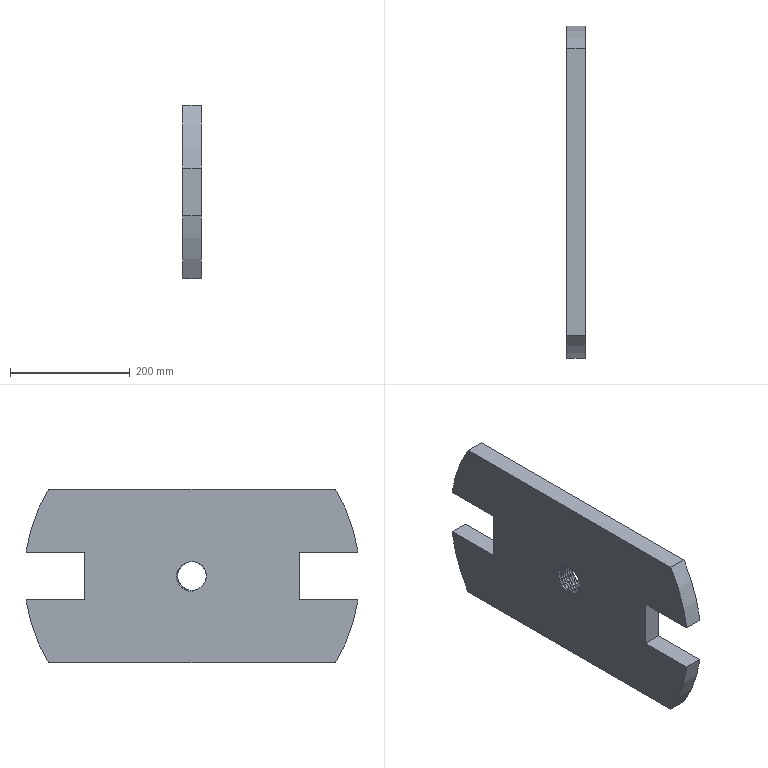Part | NX | features DATUM_CSYS 2, EXTRUDE 2, DATUM_PLANE 1, HELIX 1, SKETCH 1, SWP104 1 | 1 solid | 129 faces | box 31 x 554.256 x 290 mm | volume 4245966 mm3 | torus 113 | plane 11 | cylinder 5 | commonest cylinder face diameters 560 x4 48 x1